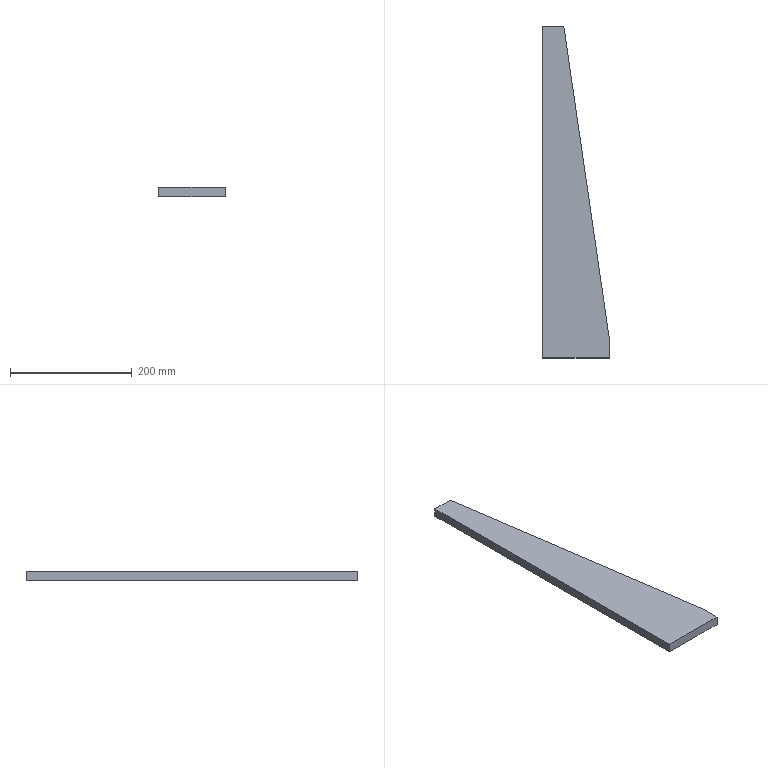Part | STEP file | 001-003-Storage mechanism rib plate | 1 solid | 7 faces | box 110 x 546 x 15 mm | volume 610650 mm3 | plane 7
STEP:
#1=CARTESIAN_POINT('',(0.,0.,0.));
#2=DIRECTION('',(0.,0.,1.));
#3=DIRECTION('',(1.,0.,0.));
#4=AXIS2_PLACEMENT_3D('',#1,#2,#3);
#5=CARTESIAN_POINT('',(55.,-273.,0.));
#6=VERTEX_POINT('',#5);
#7=CARTESIAN_POINT('',(55.,-243.,0.));
#8=VERTEX_POINT('',#7);
#9=CARTESIAN_POINT('',(55.,-273.,0.));
#10=DIRECTION('',(0.,1.,0.));
#11=VECTOR('',#10,1.);
#12=LINE('',#9,#11);
#13=CARTESIAN_POINT('',(55.,-273.,15.));
#14=DIRECTION('',(-1.,0.,0.));
#15=DIRECTION('',(0.,0.,1.));
#16=AXIS2_PLACEMENT_3D('',#13,#14,#15);
#17=PLANE('',#16);
#18=CARTESIAN_POINT('',(-15.,0.));
#19=DIRECTION('',(0.,1.));
#20=VECTOR('',#19,1.);
#21=LINE('',#18,#20);
#22=(GEOMETRIC_REPRESENTATION_CONTEXT(2)PARAMETRIC_REPRESENTATION_CONTEXT()REPRESENTATION_CONTEXT('',''));
#23=DEFINITIONAL_REPRESENTATION('',(#21),#22);
#24=PCURVE('',#17,#23);
#25=CARTESIAN_POINT('',(0.,0.,0.));
#26=DIRECTION('',(0.,0.,-1.));
#27=DIRECTION('',(-1.,0.,0.));
#28=AXIS2_PLACEMENT_3D('',#25,#26,#27);
#29=PLANE('',#28);
#30=CARTESIAN_POINT('',(-55.,-273.));
#31=DIRECTION('',(0.,1.));
#32=VECTOR('',#31,1.);
#33=LINE('',#30,#32);
#34=(GEOMETRIC_REPRESENTATION_CONTEXT(2)PARAMETRIC_REPRESENTATION_CONTEXT()REPRESENTATION_CONTEXT('',''));
#35=DEFINITIONAL_REPRESENTATION('',(#33),#34);
#36=PCURVE('',#29,#35);
#37=SURFACE_CURVE('',#12,(#24,#36),.PCURVE_S1.);
#38=EDGE_CURVE('',#6,#8,#37,.T.);
#39=ORIENTED_EDGE('',*,*,#38,.T.);
#40=CARTESIAN_POINT('',(55.,-243.,15.));
#41=VERTEX_POINT('',#40);
#42=CARTESIAN_POINT('',(55.,-243.,15.));
#43=DIRECTION('',(0.,0.,1.));
#44=VECTOR('',#43,1.);
#45=LINE('',#42,#44);
#46=CARTESIAN_POINT('',(0.,30.));
#47=DIRECTION('',(1.,0.));
#48=VECTOR('',#47,1.);
#49=LINE('',#46,#48);
#50=(GEOMETRIC_REPRESENTATION_CONTEXT(2)PARAMETRIC_REPRESENTATION_CONTEXT()REPRESENTATION_CONTEXT('',''));
#51=DEFINITIONAL_REPRESENTATION('',(#49),#50);
#52=PCURVE('',#17,#51);
#53=CARTESIAN_POINT('',(-20.,273.,15.));
#54=DIRECTION('',(-0.9896,-0.1438,0.));
#55=DIRECTION('',(0.,0.,-1.));
#56=AXIS2_PLACEMENT_3D('',#53,#54,#55);
#57=PLANE('',#56);
#58=CARTESIAN_POINT('',(0.,521.422));
#59=DIRECTION('',(-1.,0.));
#60=VECTOR('',#59,1.);
#61=LINE('',#58,#60);
#62=(GEOMETRIC_REPRESENTATION_CONTEXT(2)PARAMETRIC_REPRESENTATION_CONTEXT()REPRESENTATION_CONTEXT('',''));
#63=DEFINITIONAL_REPRESENTATION('',(#61),#62);
#64=PCURVE('',#57,#63);
#65=SURFACE_CURVE('',#45,(#52,#64),.PCURVE_S1.);
#66=EDGE_CURVE('',#8,#41,#65,.T.);
#67=ORIENTED_EDGE('',*,*,#66,.T.);
#68=CARTESIAN_POINT('',(55.,-273.,15.));
#69=VERTEX_POINT('',#68);
#70=CARTESIAN_POINT('',(55.,-273.,15.));
#71=DIRECTION('',(0.,1.,0.));
#72=VECTOR('',#71,1.);
#73=LINE('',#70,#72);
#74=CARTESIAN_POINT('',(0.,0.));
#75=DIRECTION('',(0.,1.));
#76=VECTOR('',#75,1.);
#77=LINE('',#74,#76);
#78=(GEOMETRIC_REPRESENTATION_CONTEXT(2)PARAMETRIC_REPRESENTATION_CONTEXT()REPRESENTATION_CONTEXT('',''));
#79=DEFINITIONAL_REPRESENTATION('',(#77),#78);
#80=PCURVE('',#17,#79);
#81=CARTESIAN_POINT('',(0.,0.,15.));
#82=DIRECTION('',(0.,0.,-1.));
#83=DIRECTION('',(-1.,0.,0.));
#84=AXIS2_PLACEMENT_3D('',#81,#82,#83);
#85=PLANE('',#84);
#86=CARTESIAN_POINT('',(-55.,-273.));
#87=DIRECTION('',(0.,1.));
#88=VECTOR('',#87,1.);
#89=LINE('',#86,#88);
#90=(GEOMETRIC_REPRESENTATION_CONTEXT(2)PARAMETRIC_REPRESENTATION_CONTEXT()REPRESENTATION_CONTEXT('',''));
#91=DEFINITIONAL_REPRESENTATION('',(#89),#90);
#92=PCURVE('',#85,#91);
#93=SURFACE_CURVE('',#73,(#80,#92),.PCURVE_S1.);
#94=EDGE_CURVE('',#69,#41,#93,.T.);
#95=ORIENTED_EDGE('',*,*,#94,.F.);
#96=CARTESIAN_POINT('',(55.,-273.,15.));
#97=DIRECTION('',(0.,0.,-1.));
#98=VECTOR('',#97,1.);
#99=LINE('',#96,#98);
#100=CARTESIAN_POINT('',(0.,0.));
#101=DIRECTION('',(-1.,0.));
#102=VECTOR('',#101,1.);
#103=LINE('',#100,#102);
#104=(GEOMETRIC_REPRESENTATION_CONTEXT(2)PARAMETRIC_REPRESENTATION_CONTEXT()REPRESENTATION_CONTEXT('',''));
#105=DEFINITIONAL_REPRESENTATION('',(#103),#104);
#106=PCURVE('',#17,#105);
#107=CARTESIAN_POINT('',(-55.,-273.,15.));
#108=DIRECTION('',(0.,1.,0.));
#109=DIRECTION('',(0.,0.,1.));
#110=AXIS2_PLACEMENT_3D('',#107,#108,#109);
#111=PLANE('',#110);
#112=CARTESIAN_POINT('',(0.,110.));
#113=DIRECTION('',(-1.,0.));
#114=VECTOR('',#113,1.);
#115=LINE('',#112,#114);
#116=(GEOMETRIC_REPRESENTATION_CONTEXT(2)PARAMETRIC_REPRESENTATION_CONTEXT()REPRESENTATION_CONTEXT('',''));
#117=DEFINITIONAL_REPRESENTATION('',(#115),#116);
#118=PCURVE('',#111,#117);
#119=SURFACE_CURVE('',#99,(#106,#118),.PCURVE_S1.);
#120=EDGE_CURVE('',#69,#6,#119,.T.);
#121=ORIENTED_EDGE('',*,*,#120,.T.);
#122=EDGE_LOOP('',(#39,#67,#95,#121));
#123=FACE_BOUND('',#122,.T.);
#124=ADVANCED_FACE('',(#123),#17,.F.);
#125=CARTESIAN_POINT('',(-20.,273.,15.));
#126=VERTEX_POINT('',#125);
#127=CARTESIAN_POINT('',(-55.,273.,15.));
#128=VERTEX_POINT('',#127);
#129=CARTESIAN_POINT('',(-55.,273.,15.));
#130=DIRECTION('',(-1.,0.,0.));
#131=VECTOR('',#130,1.);
#132=LINE('',#129,#131);
#133=CARTESIAN_POINT('',(-55.,273.,15.));
#134=DIRECTION('',(0.,-1.,0.));
#135=DIRECTION('',(0.,0.,-1.));
#136=AXIS2_PLACEMENT_3D('',#133,#134,#135);
#137=PLANE('',#136);
#138=CARTESIAN_POINT('',(0.,0.));
#139=DIRECTION('',(0.,-1.));
#140=VECTOR('',#139,1.);
#141=LINE('',#138,#140);
#142=(GEOMETRIC_REPRESENTATION_CONTEXT(2)PARAMETRIC_REPRESENTATION_CONTEXT()REPRESENTATION_CONTEXT('',''));
#143=DEFINITIONAL_REPRESENTATION('',(#141),#142);
#144=PCURVE('',#137,#143);
#145=CARTESIAN_POINT('',(55.,273.));
#146=DIRECTION('',(1.,0.));
#147=VECTOR('',#146,1.);
#148=LINE('',#145,#147);
#149=(GEOMETRIC_REPRESENTATION_CONTEXT(2)PARAMETRIC_REPRESENTATION_CONTEXT()REPRESENTATION_CONTEXT('',''));
#150=DEFINITIONAL_REPRESENTATION('',(#148),#149);
#151=PCURVE('',#85,#150);
#152=SURFACE_CURVE('',#132,(#144,#151),.PCURVE_S1.);
#153=EDGE_CURVE('',#126,#128,#152,.T.);
#154=ORIENTED_EDGE('',*,*,#153,.F.);
#155=CARTESIAN_POINT('',(-20.,273.,0.));
#156=VERTEX_POINT('',#155);
#157=CARTESIAN_POINT('',(-20.,273.,15.));
#158=DIRECTION('',(0.,0.,-1.));
#159=VECTOR('',#158,1.);
#160=LINE('',#157,#159);
#161=CARTESIAN_POINT('',(0.,35.));
#162=DIRECTION('',(1.,0.));
#163=VECTOR('',#162,1.);
#164=LINE('',#161,#163);
#165=(GEOMETRIC_REPRESENTATION_CONTEXT(2)PARAMETRIC_REPRESENTATION_CONTEXT()REPRESENTATION_CONTEXT('',''));
#166=DEFINITIONAL_REPRESENTATION('',(#164),#165);
#167=PCURVE('',#137,#166);
#168=CARTESIAN_POINT('',(0.,0.));
#169=DIRECTION('',(1.,0.));
#170=VECTOR('',#169,1.);
#171=LINE('',#168,#170);
#172=(GEOMETRIC_REPRESENTATION_CONTEXT(2)PARAMETRIC_REPRESENTATION_CONTEXT()REPRESENTATION_CONTEXT('',''));
#173=DEFINITIONAL_REPRESENTATION('',(#171),#172);
#174=PCURVE('',#57,#173);
#175=SURFACE_CURVE('',#160,(#167,#174),.PCURVE_S1.);
#176=EDGE_CURVE('',#126,#156,#175,.T.);
#177=ORIENTED_EDGE('',*,*,#176,.T.);
#178=CARTESIAN_POINT('',(-55.,273.,0.));
#179=VERTEX_POINT('',#178);
#180=CARTESIAN_POINT('',(-55.,273.,0.));
#181=DIRECTION('',(-1.,0.,0.));
#182=VECTOR('',#181,1.);
#183=LINE('',#180,#182);
#184=CARTESIAN_POINT('',(15.,0.));
#185=DIRECTION('',(0.,-1.));
#186=VECTOR('',#185,1.);
#187=LINE('',#184,#186);
#188=(GEOMETRIC_REPRESENTATION_CONTEXT(2)PARAMETRIC_REPRESENTATION_CONTEXT()REPRESENTATION_CONTEXT('',''));
#189=DEFINITIONAL_REPRESENTATION('',(#187),#188);
#190=PCURVE('',#137,#189);
#191=CARTESIAN_POINT('',(55.,273.));
#192=DIRECTION('',(1.,0.));
#193=VECTOR('',#192,1.);
#194=LINE('',#191,#193);
#195=(GEOMETRIC_REPRESENTATION_CONTEXT(2)PARAMETRIC_REPRESENTATION_CONTEXT()REPRESENTATION_CONTEXT('',''));
#196=DEFINITIONAL_REPRESENTATION('',(#194),#195);
#197=PCURVE('',#29,#196);
#198=SURFACE_CURVE('',#183,(#190,#197),.PCURVE_S1.);
#199=EDGE_CURVE('',#156,#179,#198,.T.);
#200=ORIENTED_EDGE('',*,*,#199,.T.);
#201=CARTESIAN_POINT('',(-55.,273.,15.));
#202=DIRECTION('',(0.,0.,-1.));
#203=VECTOR('',#202,1.);
#204=LINE('',#201,#203);
#205=CARTESIAN_POINT('',(0.,0.));
#206=DIRECTION('',(1.,0.));
#207=VECTOR('',#206,1.);
#208=LINE('',#205,#207);
#209=(GEOMETRIC_REPRESENTATION_CONTEXT(2)PARAMETRIC_REPRESENTATION_CONTEXT()REPRESENTATION_CONTEXT('',''));
#210=DEFINITIONAL_REPRESENTATION('',(#208),#209);
#211=PCURVE('',#137,#210);
#212=CARTESIAN_POINT('',(-55.,-273.,15.));
#213=DIRECTION('',(1.,0.,0.));
#214=DIRECTION('',(0.,0.,-1.));
#215=AXIS2_PLACEMENT_3D('',#212,#213,#214);
#216=PLANE('',#215);
#217=CARTESIAN_POINT('',(0.,546.));
#218=DIRECTION('',(1.,0.));
#219=VECTOR('',#218,1.);
#220=LINE('',#217,#219);
#221=(GEOMETRIC_REPRESENTATION_CONTEXT(2)PARAMETRIC_REPRESENTATION_CONTEXT()REPRESENTATION_CONTEXT('',''));
#222=DEFINITIONAL_REPRESENTATION('',(#220),#221);
#223=PCURVE('',#216,#222);
#224=SURFACE_CURVE('',#204,(#211,#223),.PCURVE_S1.);
#225=EDGE_CURVE('',#128,#179,#224,.T.);
#226=ORIENTED_EDGE('',*,*,#225,.F.);
#227=EDGE_LOOP('',(#154,#177,#200,#226));
#228=FACE_BOUND('',#227,.T.);
#229=ADVANCED_FACE('',(#228),#137,.F.);
#230=CARTESIAN_POINT('',(-55.,-273.,0.));
#231=VERTEX_POINT('',#230);
#232=CARTESIAN_POINT('',(-55.,-273.,0.));
#233=DIRECTION('',(0.,-1.,0.));
#234=VECTOR('',#233,1.);
#235=LINE('',#232,#234);
#236=CARTESIAN_POINT('',(15.,0.));
#237=DIRECTION('',(0.,-1.));
#238=VECTOR('',#237,1.);
#239=LINE('',#236,#238);
#240=(GEOMETRIC_REPRESENTATION_CONTEXT(2)PARAMETRIC_REPRESENTATION_CONTEXT()REPRESENTATION_CONTEXT('',''));
#241=DEFINITIONAL_REPRESENTATION('',(#239),#240);
#242=PCURVE('',#216,#241);
#243=CARTESIAN_POINT('',(55.,-273.));
#244=DIRECTION('',(0.,-1.));
#245=VECTOR('',#244,1.);
#246=LINE('',#243,#245);
#247=(GEOMETRIC_REPRESENTATION_CONTEXT(2)PARAMETRIC_REPRESENTATION_CONTEXT()REPRESENTATION_CONTEXT('',''));
#248=DEFINITIONAL_REPRESENTATION('',(#246),#247);
#249=PCURVE('',#29,#248);
#250=SURFACE_CURVE('',#235,(#242,#249),.PCURVE_S1.);
#251=EDGE_CURVE('',#179,#231,#250,.T.);
#252=ORIENTED_EDGE('',*,*,#251,.T.);
#253=CARTESIAN_POINT('',(-55.,-273.,15.));
#254=VERTEX_POINT('',#253);
#255=CARTESIAN_POINT('',(-55.,-273.,15.));
#256=DIRECTION('',(0.,0.,-1.));
#257=VECTOR('',#256,1.);
#258=LINE('',#255,#257);
#259=CARTESIAN_POINT('',(0.,0.));
#260=DIRECTION('',(1.,0.));
#261=VECTOR('',#260,1.);
#262=LINE('',#259,#261);
#263=(GEOMETRIC_REPRESENTATION_CONTEXT(2)PARAMETRIC_REPRESENTATION_CONTEXT()REPRESENTATION_CONTEXT('',''));
#264=DEFINITIONAL_REPRESENTATION('',(#262),#263);
#265=PCURVE('',#216,#264);
#266=CARTESIAN_POINT('',(0.,0.));
#267=DIRECTION('',(-1.,0.));
#268=VECTOR('',#267,1.);
#269=LINE('',#266,#268);
#270=(GEOMETRIC_REPRESENTATION_CONTEXT(2)PARAMETRIC_REPRESENTATION_CONTEXT()REPRESENTATION_CONTEXT('',''));
#271=DEFINITIONAL_REPRESENTATION('',(#269),#270);
#272=PCURVE('',#111,#271);
#273=SURFACE_CURVE('',#258,(#265,#272),.PCURVE_S1.);
#274=EDGE_CURVE('',#254,#231,#273,.T.);
#275=ORIENTED_EDGE('',*,*,#274,.F.);
#276=CARTESIAN_POINT('',(-55.,-273.,15.));
#277=DIRECTION('',(0.,-1.,0.));
#278=VECTOR('',#277,1.);
#279=LINE('',#276,#278);
#280=CARTESIAN_POINT('',(0.,0.));
#281=DIRECTION('',(0.,-1.));
#282=VECTOR('',#281,1.);
#283=LINE('',#280,#282);
#284=(GEOMETRIC_REPRESENTATION_CONTEXT(2)PARAMETRIC_REPRESENTATION_CONTEXT()REPRESENTATION_CONTEXT('',''));
#285=DEFINITIONAL_REPRESENTATION('',(#283),#284);
#286=PCURVE('',#216,#285);
#287=CARTESIAN_POINT('',(55.,-273.));
#288=DIRECTION('',(0.,-1.));
#289=VECTOR('',#288,1.);
#290=LINE('',#287,#289);
#291=(GEOMETRIC_REPRESENTATION_CONTEXT(2)PARAMETRIC_REPRESENTATION_CONTEXT()REPRESENTATION_CONTEXT('',''));
#292=DEFINITIONAL_REPRESENTATION('',(#290),#291);
#293=PCURVE('',#85,#292);
#294=SURFACE_CURVE('',#279,(#286,#293),.PCURVE_S1.);
#295=EDGE_CURVE('',#128,#254,#294,.T.);
#296=ORIENTED_EDGE('',*,*,#295,.F.);
#297=ORIENTED_EDGE('',*,*,#225,.T.);
#298=EDGE_LOOP('',(#252,#275,#296,#297));
#299=FACE_BOUND('',#298,.T.);
#300=ADVANCED_FACE('',(#299),#216,.F.);
#301=CARTESIAN_POINT('',(-55.,-273.,0.));
#302=DIRECTION('',(1.,0.,0.));
#303=VECTOR('',#302,1.);
#304=LINE('',#301,#303);
#305=CARTESIAN_POINT('',(-15.,0.));
#306=DIRECTION('',(0.,1.));
#307=VECTOR('',#306,1.);
#308=LINE('',#305,#307);
#309=(GEOMETRIC_REPRESENTATION_CONTEXT(2)PARAMETRIC_REPRESENTATION_CONTEXT()REPRESENTATION_CONTEXT('',''));
#310=DEFINITIONAL_REPRESENTATION('',(#308),#309);
#311=PCURVE('',#111,#310);
#312=CARTESIAN_POINT('',(55.,-273.));
#313=DIRECTION('',(-1.,0.));
#314=VECTOR('',#313,1.);
#315=LINE('',#312,#314);
#316=(GEOMETRIC_REPRESENTATION_CONTEXT(2)PARAMETRIC_REPRESENTATION_CONTEXT()REPRESENTATION_CONTEXT('',''));
#317=DEFINITIONAL_REPRESENTATION('',(#315),#316);
#318=PCURVE('',#29,#317);
#319=SURFACE_CURVE('',#304,(#311,#318),.PCURVE_S1.);
#320=EDGE_CURVE('',#231,#6,#319,.T.);
#321=ORIENTED_EDGE('',*,*,#320,.T.);
#322=ORIENTED_EDGE('',*,*,#120,.F.);
#323=CARTESIAN_POINT('',(-55.,-273.,15.));
#324=DIRECTION('',(1.,0.,0.));
#325=VECTOR('',#324,1.);
#326=LINE('',#323,#325);
#327=CARTESIAN_POINT('',(0.,0.));
#328=DIRECTION('',(0.,1.));
#329=VECTOR('',#328,1.);
#330=LINE('',#327,#329);
#331=(GEOMETRIC_REPRESENTATION_CONTEXT(2)PARAMETRIC_REPRESENTATION_CONTEXT()REPRESENTATION_CONTEXT('',''));
#332=DEFINITIONAL_REPRESENTATION('',(#330),#331);
#333=PCURVE('',#111,#332);
#334=CARTESIAN_POINT('',(55.,-273.));
#335=DIRECTION('',(-1.,0.));
#336=VECTOR('',#335,1.);
#337=LINE('',#334,#336);
#338=(GEOMETRIC_REPRESENTATION_CONTEXT(2)PARAMETRIC_REPRESENTATION_CONTEXT()REPRESENTATION_CONTEXT('',''));
#339=DEFINITIONAL_REPRESENTATION('',(#337),#338);
#340=PCURVE('',#85,#339);
#341=SURFACE_CURVE('',#326,(#333,#340),.PCURVE_S1.);
#342=EDGE_CURVE('',#254,#69,#341,.T.);
#343=ORIENTED_EDGE('',*,*,#342,.F.);
#344=ORIENTED_EDGE('',*,*,#274,.T.);
#345=EDGE_LOOP('',(#321,#322,#343,#344));
#346=FACE_BOUND('',#345,.T.);
#347=ADVANCED_FACE('',(#346),#111,.F.);
#348=ORIENTED_EDGE('',*,*,#94,.T.);
#349=CARTESIAN_POINT('',(-20.,273.,15.));
#350=DIRECTION('',(-0.1438,0.9896,0.));
#351=VECTOR('',#350,1.);
#352=LINE('',#349,#351);
#353=CARTESIAN_POINT('',(20.,273.));
#354=DIRECTION('',(0.1438,0.9896));
#355=VECTOR('',#354,1.);
#356=LINE('',#353,#355);
#357=(GEOMETRIC_REPRESENTATION_CONTEXT(2)PARAMETRIC_REPRESENTATION_CONTEXT()REPRESENTATION_CONTEXT('',''));
#358=DEFINITIONAL_REPRESENTATION('',(#356),#357);
#359=PCURVE('',#85,#358);
#360=CARTESIAN_POINT('',(0.,0.));
#361=DIRECTION('',(0.,-1.));
#362=VECTOR('',#361,1.);
#363=LINE('',#360,#362);
#364=(GEOMETRIC_REPRESENTATION_CONTEXT(2)PARAMETRIC_REPRESENTATION_CONTEXT()REPRESENTATION_CONTEXT('',''));
#365=DEFINITIONAL_REPRESENTATION('',(#363),#364);
#366=PCURVE('',#57,#365);
#367=SURFACE_CURVE('',#352,(#359,#366),.PCURVE_S1.);
#368=EDGE_CURVE('',#41,#126,#367,.T.);
#369=ORIENTED_EDGE('',*,*,#368,.T.);
#370=ORIENTED_EDGE('',*,*,#153,.T.);
#371=ORIENTED_EDGE('',*,*,#295,.T.);
#372=ORIENTED_EDGE('',*,*,#342,.T.);
#373=EDGE_LOOP('',(#348,#369,#370,#371,#372));
#374=FACE_BOUND('',#373,.T.);
#375=ADVANCED_FACE('',(#374),#85,.F.);
#376=ORIENTED_EDGE('',*,*,#199,.F.);
#377=CARTESIAN_POINT('',(19.273,2.801,0.));
#378=DIRECTION('',(0.1438,-0.9896,0.));
#379=VECTOR('',#378,1.);
#380=LINE('',#377,#379);
#381=CARTESIAN_POINT('',(-19.273,2.801));
#382=DIRECTION('',(-0.1438,-0.9896));
#383=VECTOR('',#382,1.);
#384=LINE('',#381,#383);
#385=(GEOMETRIC_REPRESENTATION_CONTEXT(2)PARAMETRIC_REPRESENTATION_CONTEXT()REPRESENTATION_CONTEXT('',''));
#386=DEFINITIONAL_REPRESENTATION('',(#384),#385);
#387=PCURVE('',#29,#386);
#388=CARTESIAN_POINT('',(15.,273.038));
#389=DIRECTION('',(0.,1.));
#390=VECTOR('',#389,1.);
#391=LINE('',#388,#390);
#392=(GEOMETRIC_REPRESENTATION_CONTEXT(2)PARAMETRIC_REPRESENTATION_CONTEXT()REPRESENTATION_CONTEXT('',''));
#393=DEFINITIONAL_REPRESENTATION('',(#391),#392);
#394=PCURVE('',#57,#393);
#395=SURFACE_CURVE('',#380,(#387,#394),.PCURVE_S1.);
#396=EDGE_CURVE('',#156,#8,#395,.T.);
#397=ORIENTED_EDGE('',*,*,#396,.T.);
#398=ORIENTED_EDGE('',*,*,#38,.F.);
#399=ORIENTED_EDGE('',*,*,#320,.F.);
#400=ORIENTED_EDGE('',*,*,#251,.F.);
#401=EDGE_LOOP('',(#376,#397,#398,#399,#400));
#402=FACE_BOUND('',#401,.T.);
#403=ADVANCED_FACE('',(#402),#29,.T.);
#404=ORIENTED_EDGE('',*,*,#368,.F.);
#405=ORIENTED_EDGE('',*,*,#66,.F.);
#406=ORIENTED_EDGE('',*,*,#396,.F.);
#407=ORIENTED_EDGE('',*,*,#176,.F.);
#408=EDGE_LOOP('',(#404,#405,#406,#407));
#409=FACE_BOUND('',#408,.T.);
#410=ADVANCED_FACE('',(#409),#57,.F.);
#411=CLOSED_SHELL('',(#124,#229,#300,#347,#375,#403,#410));
#412=MANIFOLD_SOLID_BREP('',#411);
#413=(LENGTH_UNIT()NAMED_UNIT(*)SI_UNIT(.MILLI.,.METRE.));
#414=UNCERTAINTY_MEASURE_WITH_UNIT(LENGTH_MEASURE(0.0000001),#413,'','');
#415=(NAMED_UNIT(*)PLANE_ANGLE_UNIT()SI_UNIT($,.RADIAN.));
#416=(NAMED_UNIT(*)SI_UNIT($,.STERADIAN.)SOLID_ANGLE_UNIT());
#417=(GEOMETRIC_REPRESENTATION_CONTEXT(3)GLOBAL_UNCERTAINTY_ASSIGNED_CONTEXT((#414))GLOBAL_UNIT_ASSIGNED_CONTEXT((#413,#415,#416))REPRESENTATION_CONTEXT('',''));
#418=ADVANCED_BREP_SHAPE_REPRESENTATION('',(#4,#412),#417);